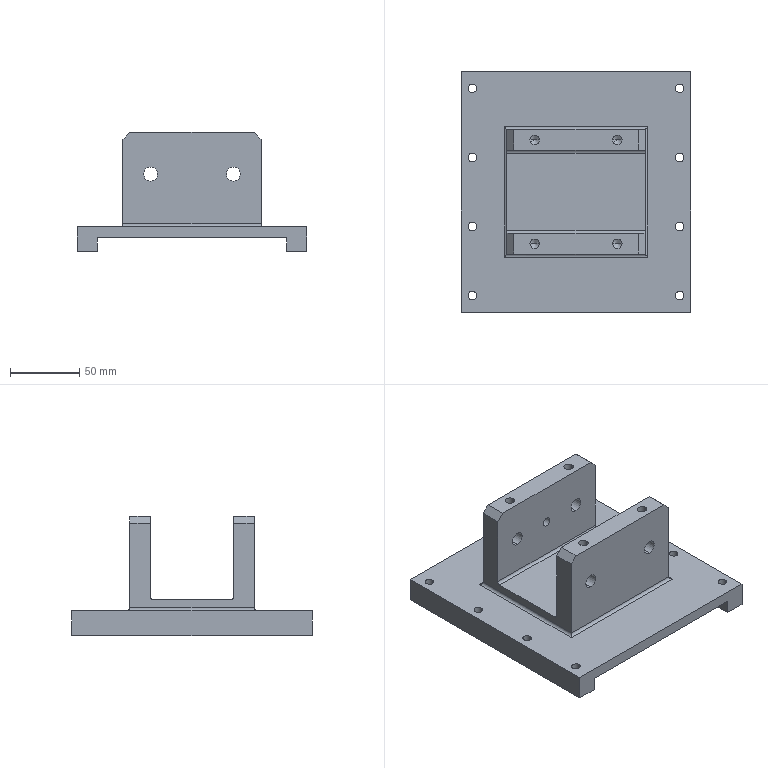Part | 1 solid | 70 faces | box 166 x 174 x 86.2 mm | volume 521198 mm3 | cylinder 39 | plane 23 | cone 8 | commonest cylinder face diameters 6.3 x16 6.8 x9 10.1 x8 4 x6